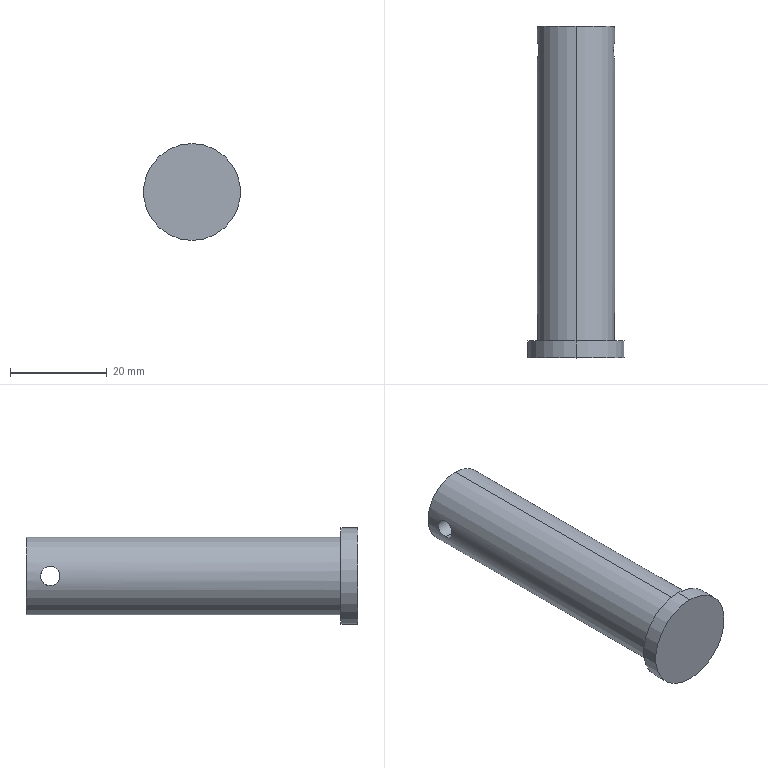Part | SolidWorks | features ICE 1, Revolution 1 | 1 solid | 9 faces | box 20 x 68.5 x 20 mm | volume 13969 mm3 | cylinder 6 | plane 3 | commonest cylinder face diameters 4 x2 16 x2 20 x2
STEP:
#1=CARTESIAN_POINT('',(-7.746,29.25,2.));
#2=VERTEX_POINT('',#1);
#3=CARTESIAN_POINT('',(-7.746,29.25,-2.));
#4=VERTEX_POINT('',#3);
#5=CARTESIAN_POINT('',(-7.746,29.25,2.));
#6=CARTESIAN_POINT('',(-7.746,28.988,2.));
#7=CARTESIAN_POINT('',(-7.76,28.724,1.947));
#8=CARTESIAN_POINT('',(-7.796,28.363,1.797));
#9=CARTESIAN_POINT('',(-7.81,28.246,1.735));
#10=CARTESIAN_POINT('',(-7.841,28.029,1.589));
#11=CARTESIAN_POINT('',(-7.857,27.929,1.507));
#12=CARTESIAN_POINT('',(-7.89,27.744,1.323));
#13=CARTESIAN_POINT('',(-7.907,27.66,1.22));
#14=CARTESIAN_POINT('',(-7.937,27.516,1.004));
#15=CARTESIAN_POINT('',(-7.951,27.454,0.8897));
#16=CARTESIAN_POINT('',(-7.987,27.302,0.5248));
#17=CARTESIAN_POINT('',(-8.,27.25,0.2644));
#18=CARTESIAN_POINT('',(-8.,27.25,-0.1313));
#19=CARTESIAN_POINT('',(-7.997,27.263,-0.2615));
#20=CARTESIAN_POINT('',(-7.984,27.314,-0.5184));
#21=CARTESIAN_POINT('',(-7.975,27.353,-0.646));
#22=CARTESIAN_POINT('',(-7.94,27.503,-1.008));
#23=CARTESIAN_POINT('',(-7.907,27.652,-1.23));
#24=CARTESIAN_POINT('',(-7.841,28.019,-1.597));
#25=CARTESIAN_POINT('',(-7.808,28.24,-1.746));
#26=CARTESIAN_POINT('',(-7.772,28.601,-1.896));
#27=CARTESIAN_POINT('',(-7.762,28.729,-1.935));
#28=CARTESIAN_POINT('',(-7.749,28.987,-1.987));
#29=CARTESIAN_POINT('',(-7.746,29.117,-2.));
#30=CARTESIAN_POINT('',(-7.746,29.25,-2.));
#31=B_SPLINE_CURVE_WITH_KNOTS('',3,(#5,#6,#7,#8,#9,#10,#11,#12,#13,#14,#15,#16,#17,#18,#19,#20,#21,#22,#23,#24,#25,#26,#27,#28,#29,#30),.UNSPECIFIED.,.F.,.F.,(4,2,2,2,2,2,2,2,2,2,2,2,4),(0.006278,0.007062,0.007455,0.007847,0.008239,0.008631,0.009416,0.009808,0.0102,0.01098,0.01177,0.01216,0.01255),.UNSPECIFIED.);
#32=EDGE_CURVE('',#2,#4,#31,.T.);
#33=ORIENTED_EDGE('',*,*,#32,.F.);
#34=CARTESIAN_POINT('',(7.746,29.25,2.));
#35=VERTEX_POINT('',#34);
#36=CARTESIAN_POINT('',(-10.,29.25,2.));
#37=DIRECTION('',(1.,0.,0.));
#38=VECTOR('',#37,1000.);
#39=LINE('',#36,#38);
#40=EDGE_CURVE('',#2,#35,#39,.T.);
#41=ORIENTED_EDGE('',*,*,#40,.T.);
#42=CARTESIAN_POINT('',(7.746,29.25,-2.));
#43=VERTEX_POINT('',#42);
#44=CARTESIAN_POINT('',(7.746,29.25,-2.));
#45=CARTESIAN_POINT('',(7.746,29.117,-2.));
#46=CARTESIAN_POINT('',(7.749,28.987,-1.987));
#47=CARTESIAN_POINT('',(7.762,28.731,-1.936));
#48=CARTESIAN_POINT('',(7.772,28.603,-1.897));
#49=CARTESIAN_POINT('',(7.796,28.361,-1.796));
#50=CARTESIAN_POINT('',(7.81,28.247,-1.735));
#51=CARTESIAN_POINT('',(7.841,28.03,-1.59));
#52=CARTESIAN_POINT('',(7.858,27.927,-1.506));
#53=CARTESIAN_POINT('',(7.907,27.652,-1.23));
#54=CARTESIAN_POINT('',(7.94,27.503,-1.008));
#55=CARTESIAN_POINT('',(7.975,27.353,-0.6471));
#56=CARTESIAN_POINT('',(7.984,27.314,-0.5204));
#57=CARTESIAN_POINT('',(7.997,27.263,-0.262));
#58=CARTESIAN_POINT('',(8.,27.25,-0.1319));
#59=CARTESIAN_POINT('',(8.,27.25,0.1302));
#60=CARTESIAN_POINT('',(7.997,27.263,0.2634));
#61=CARTESIAN_POINT('',(7.984,27.314,0.5203));
#62=CARTESIAN_POINT('',(7.975,27.352,0.6453));
#63=CARTESIAN_POINT('',(7.94,27.504,1.01));
#64=CARTESIAN_POINT('',(7.907,27.651,1.229));
#65=CARTESIAN_POINT('',(7.857,27.929,1.507));
#66=CARTESIAN_POINT('',(7.841,28.029,1.59));
#67=CARTESIAN_POINT('',(7.81,28.246,1.734));
#68=CARTESIAN_POINT('',(7.796,28.363,1.797));
#69=CARTESIAN_POINT('',(7.772,28.604,1.897));
#70=CARTESIAN_POINT('',(7.762,28.729,1.935));
#71=CARTESIAN_POINT('',(7.749,28.986,1.987));
#72=CARTESIAN_POINT('',(7.746,29.119,2.));
#73=CARTESIAN_POINT('',(7.746,29.25,2.));
#74=B_SPLINE_CURVE_WITH_KNOTS('',3,(#44,#45,#46,#47,#48,#49,#50,#51,#52,#53,#54,#55,#56,#57,#58,#59,#60,#61,#62,#63,#64,#65,#66,#67,#68,#69,#70,#71,#72,#73),.UNSPECIFIED.,.F.,.F.,(4,2,2,2,2,2,2,2,2,2,2,2,2,2,4),(0.,0.0003924,0.0007847,0.001177,0.001569,0.002354,0.002747,0.003139,0.003531,0.003924,0.004708,0.005101,0.005493,0.005885,0.006278),.UNSPECIFIED.);
#75=EDGE_CURVE('',#43,#35,#74,.T.);
#76=ORIENTED_EDGE('',*,*,#75,.F.);
#77=CARTESIAN_POINT('',(-10.,29.25,-2.));
#78=DIRECTION('',(1.,0.,0.));
#79=VECTOR('',#78,1000.);
#80=LINE('',#77,#79);
#81=EDGE_CURVE('',#4,#43,#80,.T.);
#82=ORIENTED_EDGE('',*,*,#81,.F.);
#83=EDGE_LOOP('',(#33,#41,#76,#82));
#84=FACE_OUTER_BOUND('',#83,.T.);
#85=CARTESIAN_POINT('',(-10.,29.25,0.));
#86=DIRECTION('',(1.,0.,0.));
#87=DIRECTION('',(0.,0.,-1.));
#88=AXIS2_PLACEMENT_3D('',#85,#86,#87);
#89=CYLINDRICAL_SURFACE('',#88,2.);
#90=ADVANCED_FACE('',(#84),#89,.F.);
#91=CARTESIAN_POINT('',(0.,-34.25,10.));
#92=VERTEX_POINT('',#91);
#93=CARTESIAN_POINT('',(0.,-34.25,-10.));
#94=VERTEX_POINT('',#93);
#95=CARTESIAN_POINT('',(0.,-34.25,0.));
#96=DIRECTION('',(0.,1.,0.));
#97=DIRECTION('',(0.,0.,1.));
#98=AXIS2_PLACEMENT_3D('',#95,#96,#97);
#99=CIRCLE('',#98,10.);
#100=EDGE_CURVE('',#92,#94,#99,.T.);
#101=ORIENTED_EDGE('',*,*,#100,.T.);
#102=CARTESIAN_POINT('',(0.,-30.75,-10.));
#103=VERTEX_POINT('',#102);
#104=CARTESIAN_POINT('',(0.,34.25,-10.));
#105=DIRECTION('',(0.,1.,0.));
#106=VECTOR('',#105,1000.);
#107=LINE('',#104,#106);
#108=EDGE_CURVE('',#94,#103,#107,.T.);
#109=ORIENTED_EDGE('',*,*,#108,.T.);
#110=CARTESIAN_POINT('',(0.,-30.75,10.));
#111=VERTEX_POINT('',#110);
#112=CARTESIAN_POINT('',(0.,-30.75,0.));
#113=DIRECTION('',(0.,1.,0.));
#114=DIRECTION('',(0.,0.,1.));
#115=AXIS2_PLACEMENT_3D('',#112,#113,#114);
#116=CIRCLE('',#115,10.);
#117=EDGE_CURVE('',#111,#103,#116,.T.);
#118=ORIENTED_EDGE('',*,*,#117,.F.);
#119=CARTESIAN_POINT('',(0.,34.25,10.));
#120=DIRECTION('',(0.,1.,0.));
#121=VECTOR('',#120,1000.);
#122=LINE('',#119,#121);
#123=EDGE_CURVE('',#92,#111,#122,.T.);
#124=ORIENTED_EDGE('',*,*,#123,.F.);
#125=EDGE_LOOP('',(#101,#109,#118,#124));
#126=FACE_OUTER_BOUND('',#125,.T.);
#127=CARTESIAN_POINT('',(0.,34.25,0.));
#128=DIRECTION('',(0.,1.,0.));
#129=DIRECTION('',(0.,0.,1.));
#130=AXIS2_PLACEMENT_3D('',#127,#128,#129);
#131=CYLINDRICAL_SURFACE('',#130,10.);
#132=ADVANCED_FACE('',(#126),#131,.T.);
#133=ORIENTED_EDGE('',*,*,#75,.T.);
#134=CARTESIAN_POINT('',(7.746,29.25,2.));
#135=CARTESIAN_POINT('',(7.746,29.512,2.));
#136=CARTESIAN_POINT('',(7.76,29.776,1.947));
#137=CARTESIAN_POINT('',(7.796,30.137,1.797));
#138=CARTESIAN_POINT('',(7.81,30.254,1.735));
#139=CARTESIAN_POINT('',(7.841,30.471,1.589));
#140=CARTESIAN_POINT('',(7.857,30.571,1.507));
#141=CARTESIAN_POINT('',(7.89,30.756,1.323));
#142=CARTESIAN_POINT('',(7.907,30.84,1.22));
#143=CARTESIAN_POINT('',(7.937,30.984,1.004));
#144=CARTESIAN_POINT('',(7.951,31.046,0.8897));
#145=CARTESIAN_POINT('',(7.987,31.198,0.5248));
#146=CARTESIAN_POINT('',(8.,31.25,0.2644));
#147=CARTESIAN_POINT('',(8.,31.25,-0.1313));
#148=CARTESIAN_POINT('',(7.997,31.237,-0.2615));
#149=CARTESIAN_POINT('',(7.984,31.186,-0.5184));
#150=CARTESIAN_POINT('',(7.975,31.147,-0.646));
#151=CARTESIAN_POINT('',(7.94,30.997,-1.008));
#152=CARTESIAN_POINT('',(7.907,30.848,-1.23));
#153=CARTESIAN_POINT('',(7.841,30.481,-1.597));
#154=CARTESIAN_POINT('',(7.808,30.26,-1.746));
#155=CARTESIAN_POINT('',(7.772,29.899,-1.896));
#156=CARTESIAN_POINT('',(7.762,29.771,-1.935));
#157=CARTESIAN_POINT('',(7.749,29.513,-1.987));
#158=CARTESIAN_POINT('',(7.746,29.383,-2.));
#159=CARTESIAN_POINT('',(7.746,29.25,-2.));
#160=B_SPLINE_CURVE_WITH_KNOTS('',3,(#134,#135,#136,#137,#138,#139,#140,#141,#142,#143,#144,#145,#146,#147,#148,#149,#150,#151,#152,#153,#154,#155,#156,#157,#158,#159),.UNSPECIFIED.,.F.,.F.,(4,2,2,2,2,2,2,2,2,2,2,2,4),(0.006278,0.007062,0.007455,0.007847,0.008239,0.008631,0.009416,0.009808,0.0102,0.01098,0.01177,0.01216,0.01255),.UNSPECIFIED.);
#161=EDGE_CURVE('',#35,#43,#160,.T.);
#162=ORIENTED_EDGE('',*,*,#161,.T.);
#163=EDGE_LOOP('',(#133,#162));
#164=FACE_BOUND('',#163,.T.);
#165=CARTESIAN_POINT('',(0.,-30.75,8.));
#166=VERTEX_POINT('',#165);
#167=CARTESIAN_POINT('',(0.,-30.75,-8.));
#168=VERTEX_POINT('',#167);
#169=CARTESIAN_POINT('',(0.,-30.75,0.));
#170=DIRECTION('',(0.,1.,0.));
#171=DIRECTION('',(0.,0.,1.));
#172=AXIS2_PLACEMENT_3D('',#169,#170,#171);
#173=CIRCLE('',#172,8.);
#174=EDGE_CURVE('',#166,#168,#173,.T.);
#175=ORIENTED_EDGE('',*,*,#174,.T.);
#176=CARTESIAN_POINT('',(0.,34.25,-8.));
#177=VERTEX_POINT('',#176);
#178=CARTESIAN_POINT('',(0.,34.25,-8.));
#179=DIRECTION('',(0.,1.,0.));
#180=VECTOR('',#179,1000.);
#181=LINE('',#178,#180);
#182=EDGE_CURVE('',#168,#177,#181,.T.);
#183=ORIENTED_EDGE('',*,*,#182,.T.);
#184=CARTESIAN_POINT('',(0.,34.25,8.));
#185=VERTEX_POINT('',#184);
#186=CARTESIAN_POINT('',(0.,34.25,0.));
#187=DIRECTION('',(0.,1.,0.));
#188=DIRECTION('',(0.,0.,1.));
#189=AXIS2_PLACEMENT_3D('',#186,#187,#188);
#190=CIRCLE('',#189,8.);
#191=EDGE_CURVE('',#185,#177,#190,.T.);
#192=ORIENTED_EDGE('',*,*,#191,.F.);
#193=CARTESIAN_POINT('',(0.,34.25,8.));
#194=DIRECTION('',(0.,1.,0.));
#195=VECTOR('',#194,1000.);
#196=LINE('',#193,#195);
#197=EDGE_CURVE('',#166,#185,#196,.T.);
#198=ORIENTED_EDGE('',*,*,#197,.F.);
#199=EDGE_LOOP('',(#175,#183,#192,#198));
#200=FACE_OUTER_BOUND('',#199,.T.);
#201=CARTESIAN_POINT('',(0.,34.25,0.));
#202=DIRECTION('',(0.,1.,0.));
#203=DIRECTION('',(0.,0.,1.));
#204=AXIS2_PLACEMENT_3D('',#201,#202,#203);
#205=CYLINDRICAL_SURFACE('',#204,8.);
#206=ADVANCED_FACE('',(#164,#200),#205,.T.);
#207=ORIENTED_EDGE('',*,*,#182,.F.);
#208=CARTESIAN_POINT('',(0.,-30.75,0.));
#209=DIRECTION('',(0.,1.,0.));
#210=DIRECTION('',(0.,0.,1.));
#211=AXIS2_PLACEMENT_3D('',#208,#209,#210);
#212=CIRCLE('',#211,8.);
#213=EDGE_CURVE('',#168,#166,#212,.T.);
#214=ORIENTED_EDGE('',*,*,#213,.T.);
#215=ORIENTED_EDGE('',*,*,#197,.T.);
#216=CARTESIAN_POINT('',(0.,34.25,0.));
#217=DIRECTION('',(0.,1.,0.));
#218=DIRECTION('',(0.,0.,1.));
#219=AXIS2_PLACEMENT_3D('',#216,#217,#218);
#220=CIRCLE('',#219,8.);
#221=EDGE_CURVE('',#177,#185,#220,.T.);
#222=ORIENTED_EDGE('',*,*,#221,.F.);
#223=EDGE_LOOP('',(#207,#214,#215,#222));
#224=FACE_OUTER_BOUND('',#223,.T.);
#225=CARTESIAN_POINT('',(-7.746,29.25,-2.));
#226=CARTESIAN_POINT('',(-7.746,29.383,-2.));
#227=CARTESIAN_POINT('',(-7.749,29.513,-1.987));
#228=CARTESIAN_POINT('',(-7.762,29.769,-1.936));
#229=CARTESIAN_POINT('',(-7.772,29.897,-1.897));
#230=CARTESIAN_POINT('',(-7.796,30.139,-1.796));
#231=CARTESIAN_POINT('',(-7.81,30.253,-1.735));
#232=CARTESIAN_POINT('',(-7.841,30.47,-1.59));
#233=CARTESIAN_POINT('',(-7.858,30.573,-1.506));
#234=CARTESIAN_POINT('',(-7.907,30.848,-1.23));
#235=CARTESIAN_POINT('',(-7.94,30.997,-1.008));
#236=CARTESIAN_POINT('',(-7.975,31.147,-0.6471));
#237=CARTESIAN_POINT('',(-7.984,31.186,-0.5204));
#238=CARTESIAN_POINT('',(-7.997,31.237,-0.262));
#239=CARTESIAN_POINT('',(-8.,31.25,-0.1319));
#240=CARTESIAN_POINT('',(-8.,31.25,0.1302));
#241=CARTESIAN_POINT('',(-7.997,31.237,0.2634));
#242=CARTESIAN_POINT('',(-7.984,31.186,0.5203));
#243=CARTESIAN_POINT('',(-7.975,31.148,0.6453));
#244=CARTESIAN_POINT('',(-7.94,30.996,1.01));
#245=CARTESIAN_POINT('',(-7.907,30.849,1.229));
#246=CARTESIAN_POINT('',(-7.857,30.571,1.507));
#247=CARTESIAN_POINT('',(-7.841,30.471,1.59));
#248=CARTESIAN_POINT('',(-7.81,30.254,1.734));
#249=CARTESIAN_POINT('',(-7.796,30.137,1.797));
#250=CARTESIAN_POINT('',(-7.772,29.896,1.897));
#251=CARTESIAN_POINT('',(-7.762,29.771,1.935));
#252=CARTESIAN_POINT('',(-7.749,29.514,1.987));
#253=CARTESIAN_POINT('',(-7.746,29.381,2.));
#254=CARTESIAN_POINT('',(-7.746,29.25,2.));
#255=B_SPLINE_CURVE_WITH_KNOTS('',3,(#225,#226,#227,#228,#229,#230,#231,#232,#233,#234,#235,#236,#237,#238,#239,#240,#241,#242,#243,#244,#245,#246,#247,#248,#249,#250,#251,#252,#253,#254),.UNSPECIFIED.,.F.,.F.,(4,2,2,2,2,2,2,2,2,2,2,2,2,2,4),(0.,0.0003924,0.0007847,0.001177,0.001569,0.002354,0.002747,0.003139,0.003531,0.003924,0.004708,0.005101,0.005493,0.005885,0.006278),.UNSPECIFIED.);
#256=EDGE_CURVE('',#4,#2,#255,.T.);
#257=ORIENTED_EDGE('',*,*,#256,.T.);
#258=ORIENTED_EDGE('',*,*,#32,.T.);
#259=EDGE_LOOP('',(#257,#258));
#260=FACE_BOUND('',#259,.T.);
#261=CARTESIAN_POINT('',(0.,34.25,0.));
#262=DIRECTION('',(0.,1.,0.));
#263=DIRECTION('',(0.,0.,1.));
#264=AXIS2_PLACEMENT_3D('',#261,#262,#263);
#265=CYLINDRICAL_SURFACE('',#264,8.);
#266=ADVANCED_FACE('',(#224,#260),#265,.T.);
#267=ORIENTED_EDGE('',*,*,#191,.T.);
#268=ORIENTED_EDGE('',*,*,#221,.T.);
#269=EDGE_LOOP('',(#267,#268));
#270=FACE_OUTER_BOUND('',#269,.T.);
#271=CARTESIAN_POINT('',(8.,34.25,0.));
#272=DIRECTION('',(0.,-1.,0.));
#273=DIRECTION('',(0.,0.,-1.));
#274=AXIS2_PLACEMENT_3D('',#271,#272,#273);
#275=PLANE('',#274);
#276=ADVANCED_FACE('',(#270),#275,.F.);
#277=ORIENTED_EDGE('',*,*,#100,.F.);
#278=CARTESIAN_POINT('',(0.,-34.25,0.));
#279=DIRECTION('',(0.,1.,0.));
#280=DIRECTION('',(0.,0.,1.));
#281=AXIS2_PLACEMENT_3D('',#278,#279,#280);
#282=CIRCLE('',#281,10.);
#283=EDGE_CURVE('',#94,#92,#282,.T.);
#284=ORIENTED_EDGE('',*,*,#283,.F.);
#285=EDGE_LOOP('',(#277,#284));
#286=FACE_OUTER_BOUND('',#285,.T.);
#287=CARTESIAN_POINT('',(0.,-34.25,0.));
#288=DIRECTION('',(0.,1.,0.));
#289=DIRECTION('',(0.,0.,1.));
#290=AXIS2_PLACEMENT_3D('',#287,#288,#289);
#291=PLANE('',#290);
#292=ADVANCED_FACE('',(#286),#291,.F.);
#293=ORIENTED_EDGE('',*,*,#108,.F.);
#294=ORIENTED_EDGE('',*,*,#283,.T.);
#295=ORIENTED_EDGE('',*,*,#123,.T.);
#296=CARTESIAN_POINT('',(0.,-30.75,0.));
#297=DIRECTION('',(0.,1.,0.));
#298=DIRECTION('',(0.,0.,1.));
#299=AXIS2_PLACEMENT_3D('',#296,#297,#298);
#300=CIRCLE('',#299,10.);
#301=EDGE_CURVE('',#103,#111,#300,.T.);
#302=ORIENTED_EDGE('',*,*,#301,.F.);
#303=EDGE_LOOP('',(#293,#294,#295,#302));
#304=FACE_OUTER_BOUND('',#303,.T.);
#305=CARTESIAN_POINT('',(0.,34.25,0.));
#306=DIRECTION('',(0.,1.,0.));
#307=DIRECTION('',(0.,0.,1.));
#308=AXIS2_PLACEMENT_3D('',#305,#306,#307);
#309=CYLINDRICAL_SURFACE('',#308,10.);
#310=ADVANCED_FACE('',(#304),#309,.T.);
#311=ORIENTED_EDGE('',*,*,#174,.F.);
#312=ORIENTED_EDGE('',*,*,#213,.F.);
#313=EDGE_LOOP('',(#311,#312));
#314=FACE_BOUND('',#313,.T.);
#315=ORIENTED_EDGE('',*,*,#117,.T.);
#316=ORIENTED_EDGE('',*,*,#301,.T.);
#317=EDGE_LOOP('',(#315,#316));
#318=FACE_OUTER_BOUND('',#317,.T.);
#319=CARTESIAN_POINT('',(10.,-30.75,0.));
#320=DIRECTION('',(0.,-1.,0.));
#321=DIRECTION('',(0.,0.,-1.));
#322=AXIS2_PLACEMENT_3D('',#319,#320,#321);
#323=PLANE('',#322);
#324=ADVANCED_FACE('',(#314,#318),#323,.F.);
#325=ORIENTED_EDGE('',*,*,#40,.F.);
#326=ORIENTED_EDGE('',*,*,#256,.F.);
#327=ORIENTED_EDGE('',*,*,#81,.T.);
#328=ORIENTED_EDGE('',*,*,#161,.F.);
#329=EDGE_LOOP('',(#325,#326,#327,#328));
#330=FACE_OUTER_BOUND('',#329,.T.);
#331=CARTESIAN_POINT('',(-10.,29.25,0.));
#332=DIRECTION('',(1.,0.,0.));
#333=DIRECTION('',(0.,0.,-1.));
#334=AXIS2_PLACEMENT_3D('',#331,#332,#333);
#335=CYLINDRICAL_SURFACE('',#334,2.);
#336=ADVANCED_FACE('',(#330),#335,.F.);
#337=CLOSED_SHELL('',(#90,#132,#206,#266,#276,#292,#310,#324,#336));
#338=MANIFOLD_SOLID_BREP('',#337);
#339=CARTESIAN_POINT('',(0.,0.,0.));
#340=DIRECTION('',(0.,0.,1.));
#341=DIRECTION('',(1.,0.,0.));
#342=AXIS2_PLACEMENT_3D('',#339,#340,#341);
#343=(LENGTH_UNIT()NAMED_UNIT(*)SI_UNIT(.MILLI.,.METRE.));
#344=UNCERTAINTY_MEASURE_WITH_UNIT(LENGTH_MEASURE(0.00001),#343,'','');
#345=(NAMED_UNIT(*)PLANE_ANGLE_UNIT()SI_UNIT($,.RADIAN.));
#346=(NAMED_UNIT(*)SI_UNIT($,.STERADIAN.)SOLID_ANGLE_UNIT());
#347=(GEOMETRIC_REPRESENTATION_CONTEXT(3)GLOBAL_UNCERTAINTY_ASSIGNED_CONTEXT((#344))GLOBAL_UNIT_ASSIGNED_CONTEXT((#343,#345,#346))REPRESENTATION_CONTEXT('',''));
#348=ADVANCED_BREP_SHAPE_REPRESENTATION('',(#338,#342),#347);